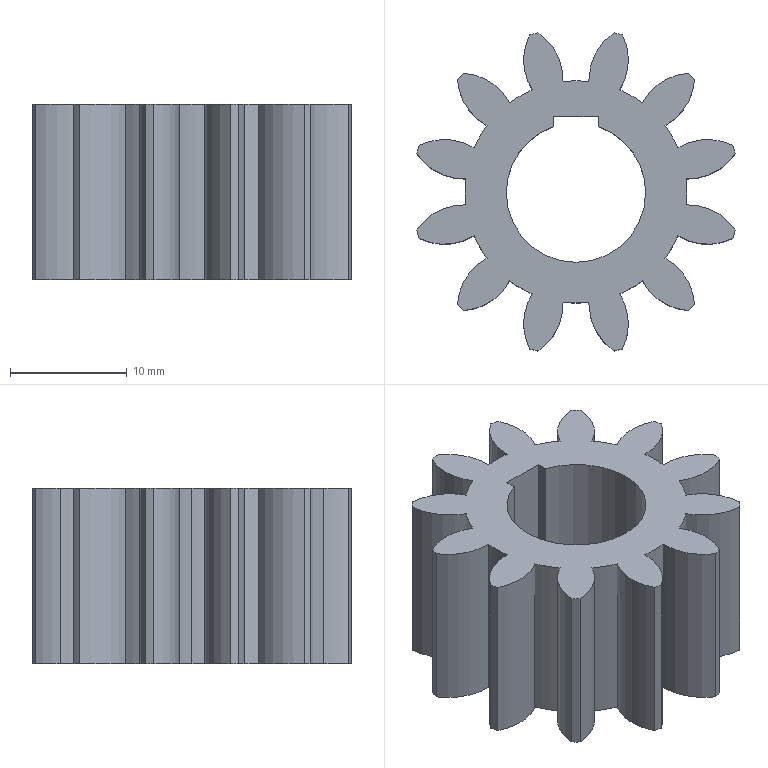Part | SolidWorks | features Extrusion 1 | 1 solid | 61 faces | box 27.226 x 27.226 x 15 mm | volume 4643 mm3 | cylinder 56 | plane 5 | commonest cylinder face diameters 9.6 x28 18.998 x13 28 x12 11.929 x3